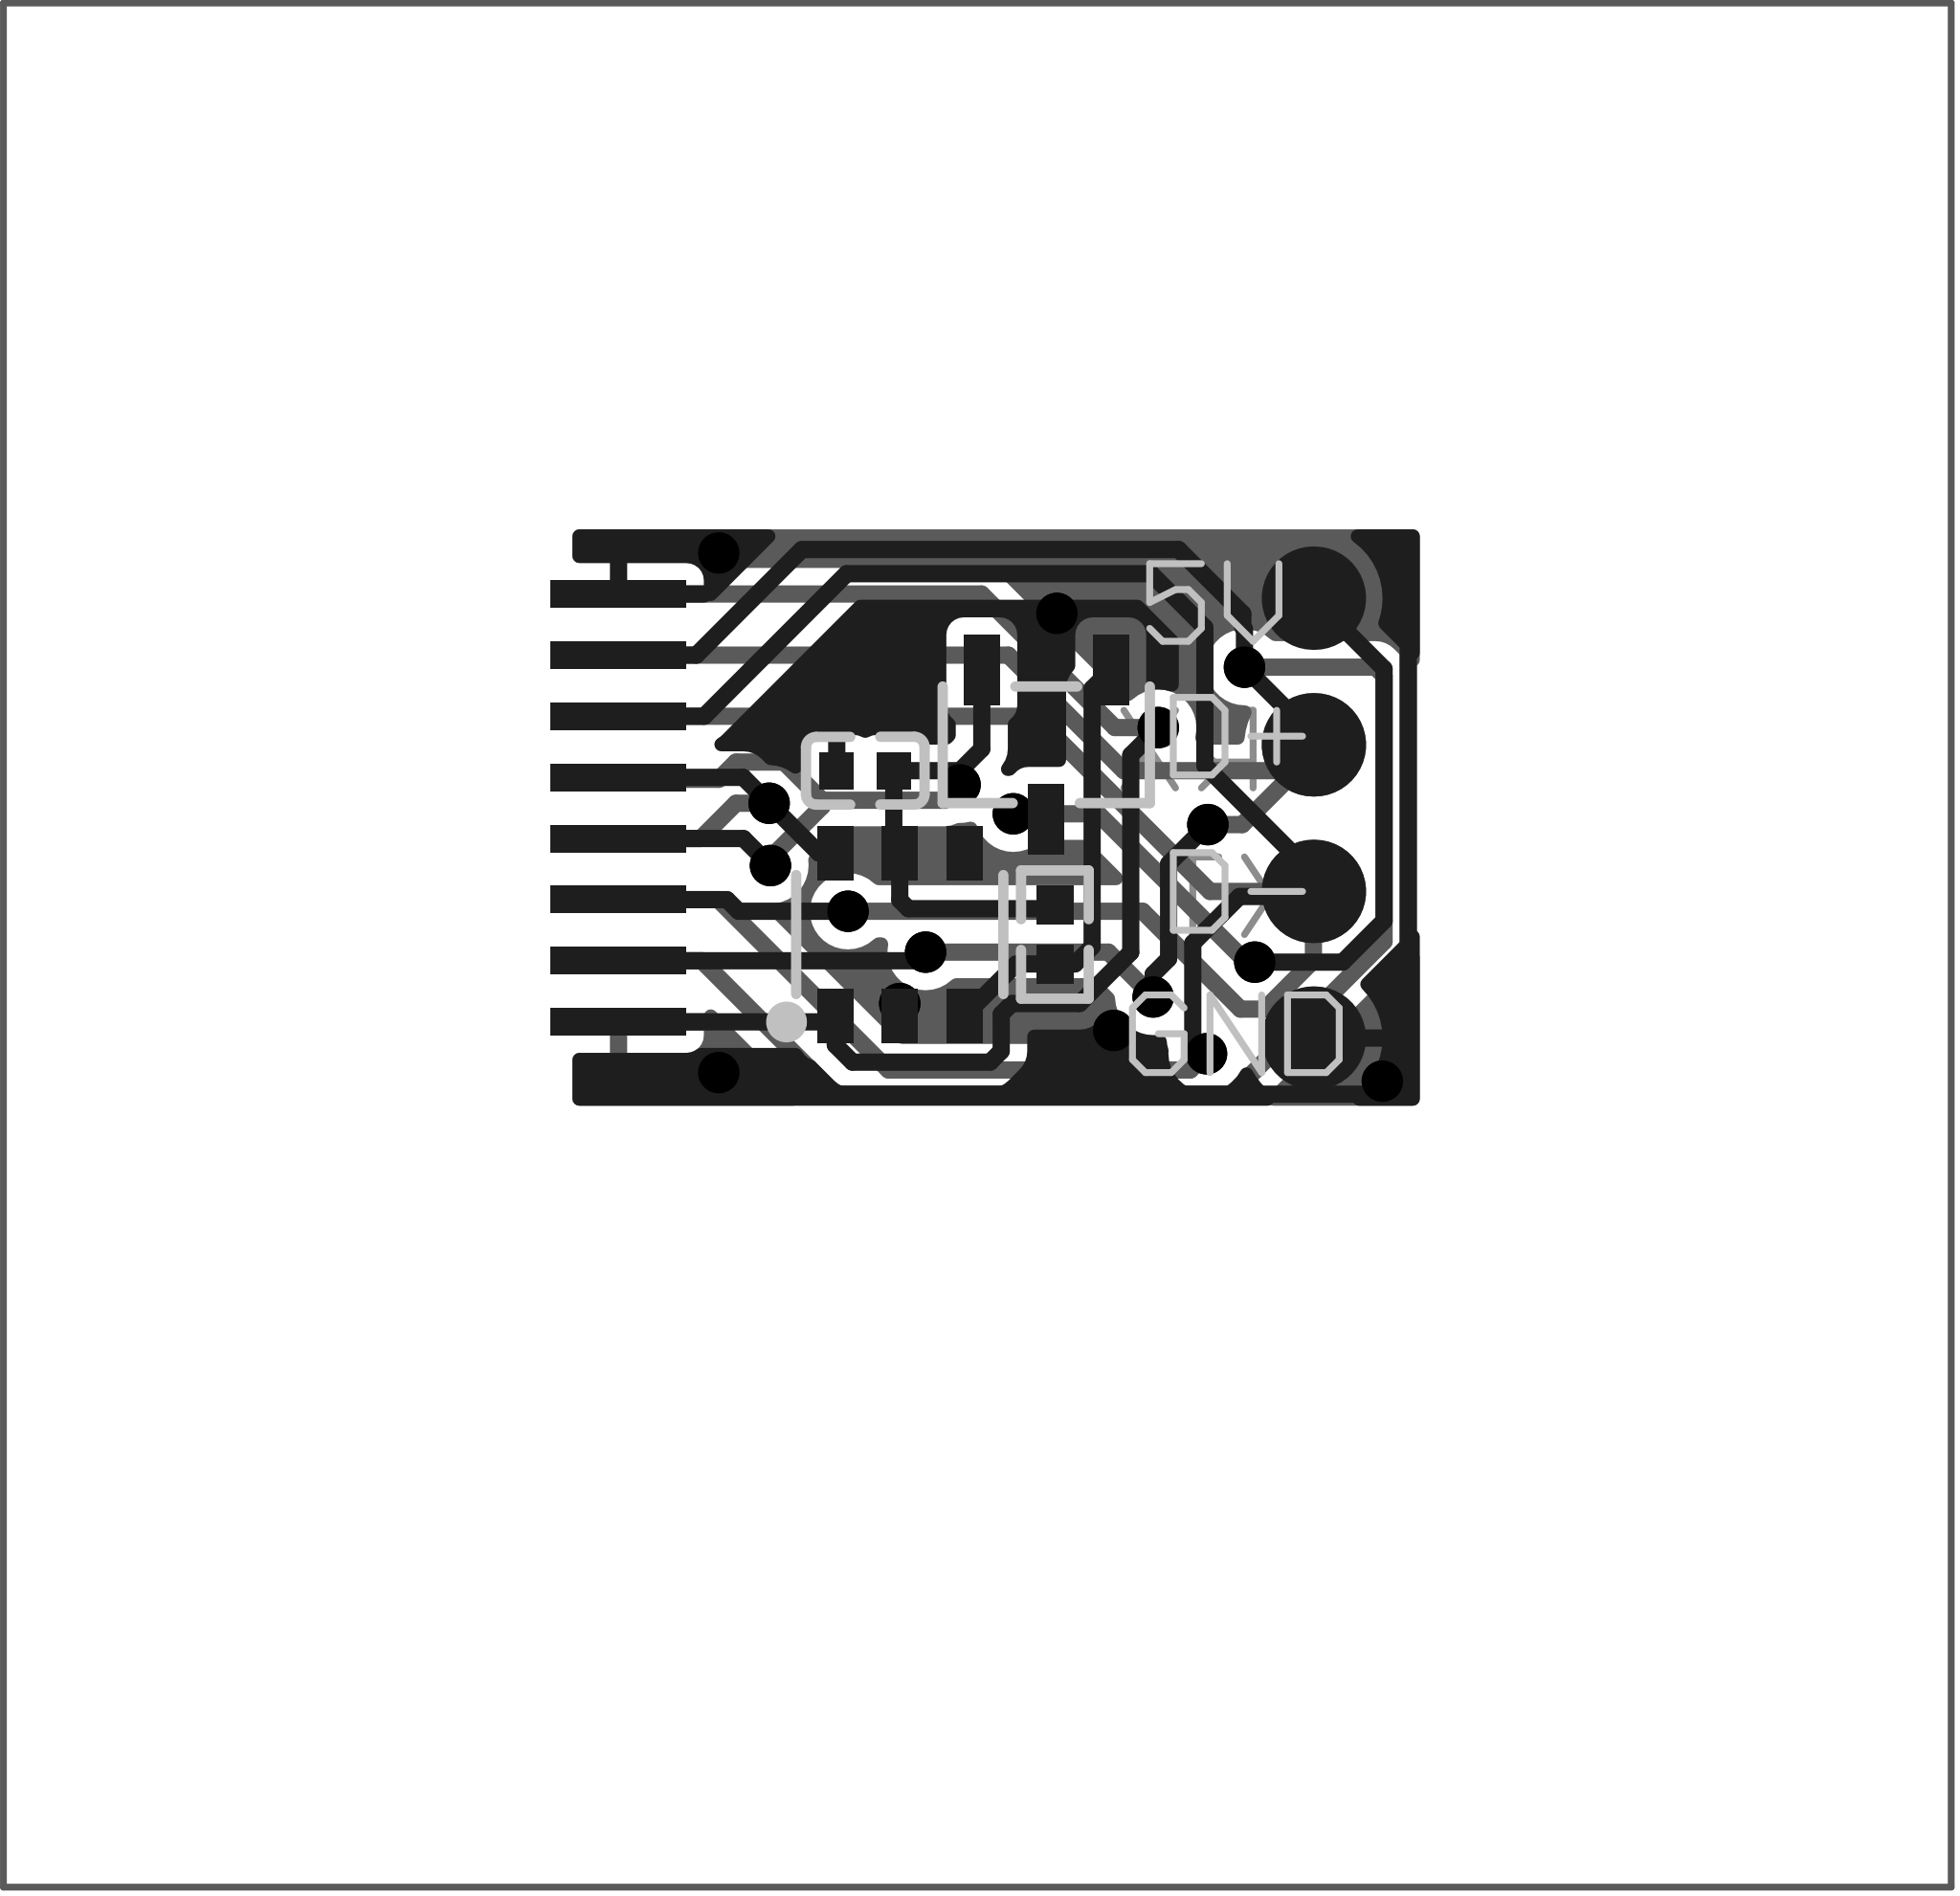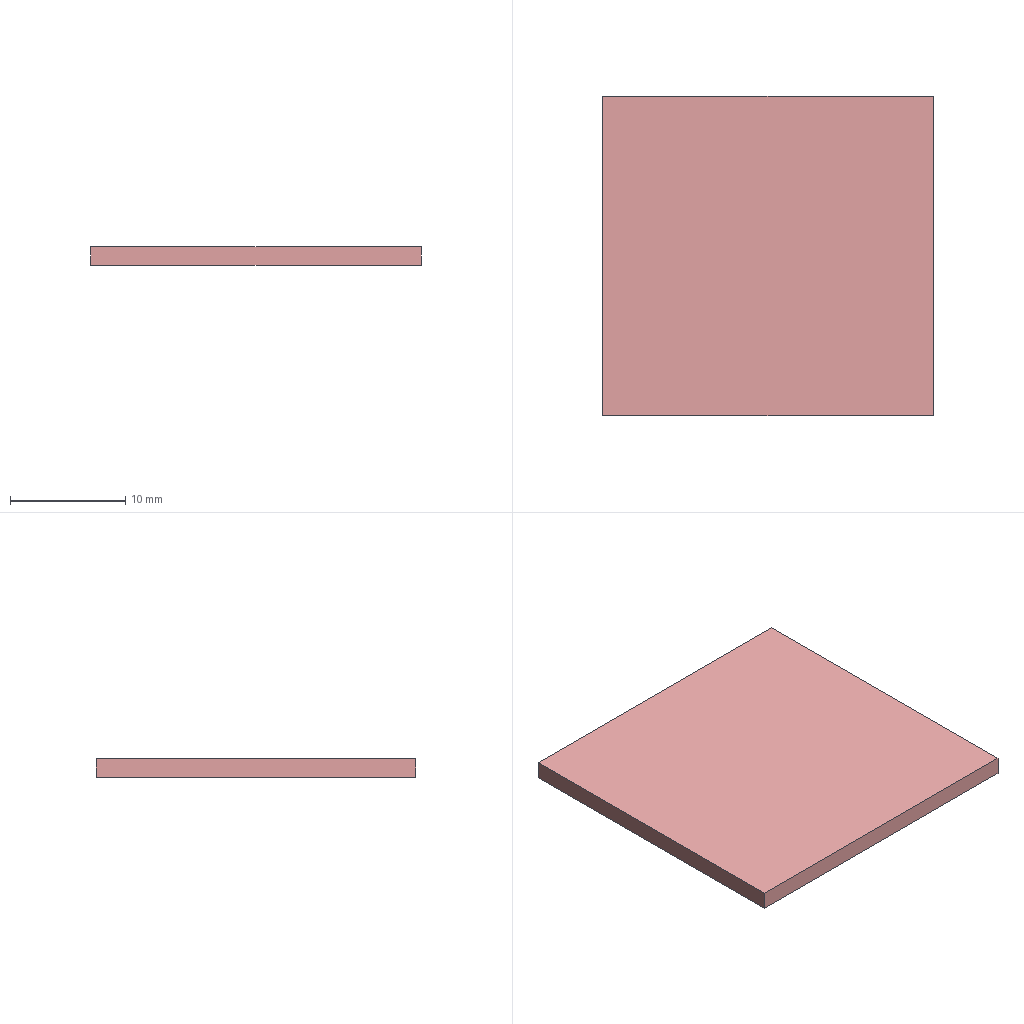Circuit board layout | Altium Designer | box 28.7 x 27.7 x 1.6 mm
Layer stack:
# Altium Designer layer stack of  (unit mm; dielectric type: 0 none, 1 core, 2 prepreg, 3 surface material)
index,name,kind,layer,copper_thickness_mm,dielectric_type,dielectric_thickness_mm,dielectric_material,dielectric_constant
0,Top Paste Mask Layer,other,,,,,,
1,Top Silkscreen Layer,other,,,,,,
2,Top Solder Mask Layer,dielectric,,,3,0.01,,3.3
3,Top Layer,copper,Top Layer,0.035,,,,
4,Dielectric1,dielectric,,,3,1.51,FR4,4.5
5,Bottom Layer,copper,Bottom Layer,0.035,,,,
6,Bottom Solder Mask Layer,dielectric,,,3,0.01,,3.3
7,Bottom Silkscreen Layer,other,,,,,,
8,Bottom Paste Mask Layer,other,,,,,,
# drill layer pairs: low layer,high layer
drill_pair,Top Layer,Bottom Layer
Part placement:
Designator,Comment,Layer,Footprint,Center-X(mm),Center-Y(mm),Rotation
C1,1uF,TopLayer,C0402,82.55,86.289,180
H1,,TopLayer,HDR-TH_16P-P2.54-V-F-R2-C8-S2.54-1,78.914,85.74,90
Q1,2301,TopLayer,SOT-23-3_L3.0-W1.7-P0.95-LS2.9-BR,85.217,86.67,90
R1,10K,TopLayer,R0402,85.344,83.876,90
U1,APS0227,TopLayer,TSOT-23-6_L2.9-W1.6-P0.95-LS2.8-BR,83.058,83.876,270
Pad and via stacks:
# Altium Designer via and pad stacks of  (unit mm). Each distinct definition once, with the count of objects using it.
# via: kind,start_layer,end_layer,hole_mm,diameter_mm,mode(0 simple;1 top-mid-bottom;2 full stack),diameter_per_layer,count,example_net
# pad: kind,layer,hole_mm,hole_type(0 round;1 square;2 slot),plating,top_size,top_shape(1 round;2 rect;3 octagon;9 rounded rect),mid_size,bottom_size,mode,footprint,size_per_layer,count,example
pad,Top Layer,0,0,plated,0.5x0.54,2,0.5x0.54,0.5x0.54,0,C0402,,2,C1.2
pad,Top Layer,0,0,plated,0.4x2,2,0.4x2,0.4x2,0,HDR-TH_16P-P2.54-V-F-R2-C8-S2.54-1,,8,H1.1
pad,Top Layer,0,0,plated,1.038x0.532,2,1.038x0.532,1.038x0.532,0,SOT-23-3_L3.0-W1.7-P0.95-LS2.9-BR,,3,Q1.1
pad,Top Layer,0,0,plated,0.5657x0.54,2,0.5657x0.54,0.5657x0.54,0,R0402,,2,R1.2
pad,Top Layer,0,0,plated,0.8x0.532,2,0.8x0.532,0.8x0.532,0,TSOT-23-6_L2.9-W1.6-P0.95-LS2.8-BR,,6,U1.1
pad,Top Layer,0,0,plated,1.524x1.524,1,1.524x1.524,1.524x1.524,0,,,4,1
pad,Bottom Layer,0,0,plated,0.4x2,2,0.4x2,0.4x2,0,HDR-TH_16P-P2.54-V-F-R2-C8-S2.54-1,,8,H1.2
pad,Bottom Layer,0,0,plated,1.524x1.524,1,1.524x1.524,1.524x1.524,0,,,2,2
via,Top Layer,Bottom Layer,0.3048,0.61,0,,18,DATA2
Copper pours:
name,layer,net,type(0 solid;1 hatched;2 none)
Bottom Layer-GND,Bottom Layer,GND,0
Top Layer-GND,Top Layer,GND,0